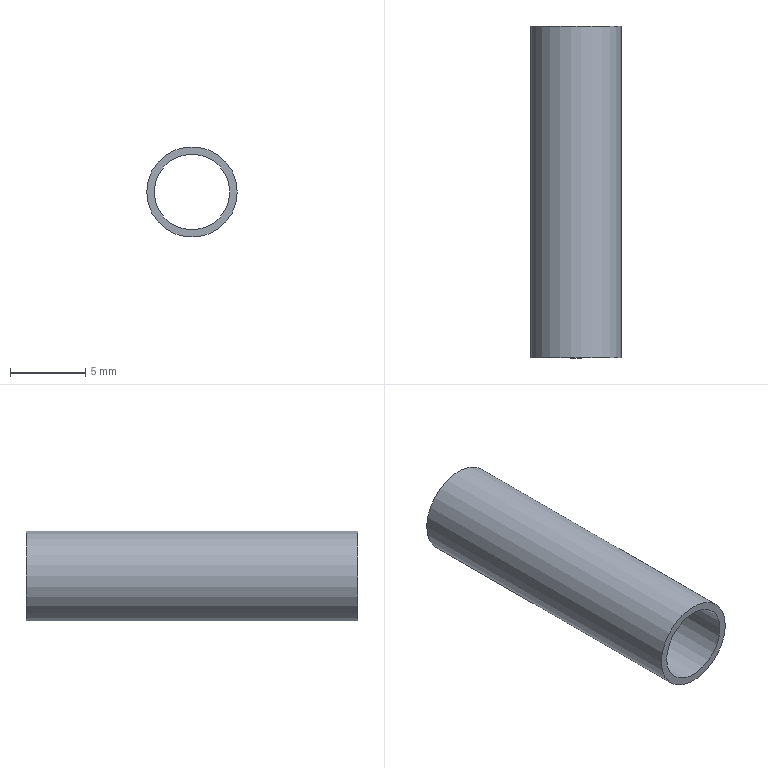Part | STEP file | 1-73.9 | 1 solid | 4 faces | box 6 x 22 x 6 mm | volume 190.066 mm3 | cylinder 2 | plane 2 | commonest cylinder face diameters 5 x1 6 x1
STEP:
#1=CARTESIAN_POINT('',(0.,0.,0.));
#2=DIRECTION('',(0.,0.,1.));
#3=DIRECTION('',(1.,0.,0.));
#4=AXIS2_PLACEMENT_3D('',#1,#2,#3);
#5=CARTESIAN_POINT('',(3.,0.,0.));
#6=VERTEX_POINT('',#5);
#7=CARTESIAN_POINT('',(0.,0.,0.));
#8=DIRECTION('',(0.,-1.,0.));
#9=DIRECTION('',(1.,0.,0.));
#10=AXIS2_PLACEMENT_3D('',#7,#8,#9);
#11=CIRCLE('',#10,3.);
#12=CARTESIAN_POINT('',(0.,0.,0.));
#13=DIRECTION('',(0.,1.,0.));
#14=DIRECTION('',(1.,0.,0.));
#15=AXIS2_PLACEMENT_3D('',#12,#13,#14);
#16=CYLINDRICAL_SURFACE('',#15,3.);
#17=CARTESIAN_POINT('',(6.283,0.));
#18=DIRECTION('',(-1.,0.));
#19=VECTOR('',#18,1.);
#20=LINE('',#17,#19);
#21=(GEOMETRIC_REPRESENTATION_CONTEXT(2)PARAMETRIC_REPRESENTATION_CONTEXT()REPRESENTATION_CONTEXT('',''));
#22=DEFINITIONAL_REPRESENTATION('',(#20),#21);
#23=PCURVE('',#16,#22);
#24=CARTESIAN_POINT('',(0.,0.,0.));
#25=DIRECTION('',(0.,-1.,0.));
#26=DIRECTION('',(0.,0.,-1.));
#27=AXIS2_PLACEMENT_3D('',#24,#25,#26);
#28=PLANE('',#27);
#29=CARTESIAN_POINT('',(0.,0.));
#30=DIRECTION('',(0.,1.));
#31=AXIS2_PLACEMENT_2D('',#29,#30);
#32=CIRCLE('',#31,3.);
#33=(GEOMETRIC_REPRESENTATION_CONTEXT(2)PARAMETRIC_REPRESENTATION_CONTEXT()REPRESENTATION_CONTEXT('',''));
#34=DEFINITIONAL_REPRESENTATION('',(#32),#33);
#35=PCURVE('',#28,#34);
#36=SURFACE_CURVE('',#11,(#23,#35),.PCURVE_S1.);
#37=EDGE_CURVE('',#6,#6,#36,.T.);
#38=ORIENTED_EDGE('',*,*,#37,.F.);
#39=CARTESIAN_POINT('',(3.,22.,0.));
#40=VERTEX_POINT('',#39);
#41=CARTESIAN_POINT('',(3.,0.,0.));
#42=DIRECTION('',(0.,1.,0.));
#43=VECTOR('',#42,1.);
#44=LINE('',#41,#43);
#45=CARTESIAN_POINT('',(6.283,0.));
#46=DIRECTION('',(0.,1.));
#47=VECTOR('',#46,1.);
#48=LINE('',#45,#47);
#49=(GEOMETRIC_REPRESENTATION_CONTEXT(2)PARAMETRIC_REPRESENTATION_CONTEXT()REPRESENTATION_CONTEXT('',''));
#50=DEFINITIONAL_REPRESENTATION('',(#48),#49);
#51=PCURVE('',#16,#50);
#52=CARTESIAN_POINT('',(0.,0.));
#53=DIRECTION('',(0.,1.));
#54=VECTOR('',#53,1.);
#55=LINE('',#52,#54);
#56=(GEOMETRIC_REPRESENTATION_CONTEXT(2)PARAMETRIC_REPRESENTATION_CONTEXT()REPRESENTATION_CONTEXT('',''));
#57=DEFINITIONAL_REPRESENTATION('',(#55),#56);
#58=PCURVE('',#16,#57);
#59=SEAM_CURVE('',#44,(#51,#58),.PCURVE_S1.);
#60=EDGE_CURVE('',#6,#40,#59,.T.);
#61=ORIENTED_EDGE('',*,*,#60,.T.);
#62=CARTESIAN_POINT('',(0.,22.,0.));
#63=DIRECTION('',(0.,1.,0.));
#64=DIRECTION('',(1.,0.,0.));
#65=AXIS2_PLACEMENT_3D('',#62,#63,#64);
#66=CIRCLE('',#65,3.);
#67=CARTESIAN_POINT('',(0.,22.));
#68=DIRECTION('',(1.,0.));
#69=VECTOR('',#68,1.);
#70=LINE('',#67,#69);
#71=(GEOMETRIC_REPRESENTATION_CONTEXT(2)PARAMETRIC_REPRESENTATION_CONTEXT()REPRESENTATION_CONTEXT('',''));
#72=DEFINITIONAL_REPRESENTATION('',(#70),#71);
#73=PCURVE('',#16,#72);
#74=CARTESIAN_POINT('',(0.,22.,0.));
#75=DIRECTION('',(0.,1.,0.));
#76=DIRECTION('',(0.,0.,1.));
#77=AXIS2_PLACEMENT_3D('',#74,#75,#76);
#78=PLANE('',#77);
#79=CARTESIAN_POINT('',(0.,0.));
#80=DIRECTION('',(0.,1.));
#81=AXIS2_PLACEMENT_2D('',#79,#80);
#82=CIRCLE('',#81,3.);
#83=(GEOMETRIC_REPRESENTATION_CONTEXT(2)PARAMETRIC_REPRESENTATION_CONTEXT()REPRESENTATION_CONTEXT('',''));
#84=DEFINITIONAL_REPRESENTATION('',(#82),#83);
#85=PCURVE('',#78,#84);
#86=SURFACE_CURVE('',#66,(#73,#85),.PCURVE_S1.);
#87=EDGE_CURVE('',#40,#40,#86,.T.);
#88=ORIENTED_EDGE('',*,*,#87,.F.);
#89=ORIENTED_EDGE('',*,*,#60,.F.);
#90=EDGE_LOOP('',(#38,#61,#88,#89));
#91=FACE_BOUND('',#90,.T.);
#92=ADVANCED_FACE('',(#91),#16,.T.);
#93=ORIENTED_EDGE('',*,*,#37,.T.);
#94=EDGE_LOOP('',(#93));
#95=FACE_BOUND('',#94,.T.);
#96=CARTESIAN_POINT('',(2.5,0.,0.));
#97=VERTEX_POINT('',#96);
#98=CARTESIAN_POINT('',(0.,0.,0.));
#99=DIRECTION('',(0.,-1.,0.));
#100=DIRECTION('',(1.,0.,0.));
#101=AXIS2_PLACEMENT_3D('',#98,#99,#100);
#102=CIRCLE('',#101,2.5);
#103=CARTESIAN_POINT('',(0.,0.));
#104=DIRECTION('',(0.,1.));
#105=AXIS2_PLACEMENT_2D('',#103,#104);
#106=CIRCLE('',#105,2.5);
#107=(GEOMETRIC_REPRESENTATION_CONTEXT(2)PARAMETRIC_REPRESENTATION_CONTEXT()REPRESENTATION_CONTEXT('',''));
#108=DEFINITIONAL_REPRESENTATION('',(#106),#107);
#109=PCURVE('',#28,#108);
#110=CARTESIAN_POINT('',(0.,0.,0.));
#111=DIRECTION('',(0.,1.,0.));
#112=DIRECTION('',(1.,0.,0.));
#113=AXIS2_PLACEMENT_3D('',#110,#111,#112);
#114=CYLINDRICAL_SURFACE('',#113,2.5);
#115=CARTESIAN_POINT('',(6.283,0.));
#116=DIRECTION('',(-1.,0.));
#117=VECTOR('',#116,1.);
#118=LINE('',#115,#117);
#119=(GEOMETRIC_REPRESENTATION_CONTEXT(2)PARAMETRIC_REPRESENTATION_CONTEXT()REPRESENTATION_CONTEXT('',''));
#120=DEFINITIONAL_REPRESENTATION('',(#118),#119);
#121=PCURVE('',#114,#120);
#122=SURFACE_CURVE('',#102,(#109,#121),.PCURVE_S1.);
#123=EDGE_CURVE('',#97,#97,#122,.T.);
#124=ORIENTED_EDGE('',*,*,#123,.F.);
#125=EDGE_LOOP('',(#124));
#126=FACE_BOUND('',#125,.T.);
#127=ADVANCED_FACE('',(#95,#126),#28,.T.);
#128=ORIENTED_EDGE('',*,*,#87,.T.);
#129=EDGE_LOOP('',(#128));
#130=FACE_BOUND('',#129,.T.);
#131=CARTESIAN_POINT('',(2.5,22.,0.));
#132=VERTEX_POINT('',#131);
#133=CARTESIAN_POINT('',(0.,22.,0.));
#134=DIRECTION('',(0.,1.,0.));
#135=DIRECTION('',(1.,0.,0.));
#136=AXIS2_PLACEMENT_3D('',#133,#134,#135);
#137=CIRCLE('',#136,2.5);
#138=CARTESIAN_POINT('',(0.,0.));
#139=DIRECTION('',(0.,1.));
#140=AXIS2_PLACEMENT_2D('',#138,#139);
#141=CIRCLE('',#140,2.5);
#142=(GEOMETRIC_REPRESENTATION_CONTEXT(2)PARAMETRIC_REPRESENTATION_CONTEXT()REPRESENTATION_CONTEXT('',''));
#143=DEFINITIONAL_REPRESENTATION('',(#141),#142);
#144=PCURVE('',#78,#143);
#145=CARTESIAN_POINT('',(0.,22.));
#146=DIRECTION('',(1.,0.));
#147=VECTOR('',#146,1.);
#148=LINE('',#145,#147);
#149=(GEOMETRIC_REPRESENTATION_CONTEXT(2)PARAMETRIC_REPRESENTATION_CONTEXT()REPRESENTATION_CONTEXT('',''));
#150=DEFINITIONAL_REPRESENTATION('',(#148),#149);
#151=PCURVE('',#114,#150);
#152=SURFACE_CURVE('',#137,(#144,#151),.PCURVE_S1.);
#153=EDGE_CURVE('',#132,#132,#152,.T.);
#154=ORIENTED_EDGE('',*,*,#153,.F.);
#155=EDGE_LOOP('',(#154));
#156=FACE_BOUND('',#155,.T.);
#157=ADVANCED_FACE('',(#130,#156),#78,.T.);
#158=ORIENTED_EDGE('',*,*,#123,.F.);
#159=CARTESIAN_POINT('',(2.5,0.,0.));
#160=DIRECTION('',(0.,1.,0.));
#161=VECTOR('',#160,1.);
#162=LINE('',#159,#161);
#163=CARTESIAN_POINT('',(6.283,0.));
#164=DIRECTION('',(0.,1.));
#165=VECTOR('',#164,1.);
#166=LINE('',#163,#165);
#167=(GEOMETRIC_REPRESENTATION_CONTEXT(2)PARAMETRIC_REPRESENTATION_CONTEXT()REPRESENTATION_CONTEXT('',''));
#168=DEFINITIONAL_REPRESENTATION('',(#166),#167);
#169=PCURVE('',#114,#168);
#170=CARTESIAN_POINT('',(0.,0.));
#171=DIRECTION('',(0.,1.));
#172=VECTOR('',#171,1.);
#173=LINE('',#170,#172);
#174=(GEOMETRIC_REPRESENTATION_CONTEXT(2)PARAMETRIC_REPRESENTATION_CONTEXT()REPRESENTATION_CONTEXT('',''));
#175=DEFINITIONAL_REPRESENTATION('',(#173),#174);
#176=PCURVE('',#114,#175);
#177=SEAM_CURVE('',#162,(#169,#176),.PCURVE_S1.);
#178=EDGE_CURVE('',#97,#132,#177,.T.);
#179=ORIENTED_EDGE('',*,*,#178,.T.);
#180=ORIENTED_EDGE('',*,*,#153,.F.);
#181=ORIENTED_EDGE('',*,*,#178,.F.);
#182=EDGE_LOOP('',(#158,#179,#180,#181));
#183=FACE_BOUND('',#182,.F.);
#184=ADVANCED_FACE('',(#183),#114,.F.);
#185=CLOSED_SHELL('',(#92,#127,#157,#184));
#186=MANIFOLD_SOLID_BREP('',#185);
#187=(LENGTH_UNIT()NAMED_UNIT(*)SI_UNIT(.MILLI.,.METRE.));
#188=UNCERTAINTY_MEASURE_WITH_UNIT(LENGTH_MEASURE(0.0000001),#187,'','');
#189=(NAMED_UNIT(*)PLANE_ANGLE_UNIT()SI_UNIT($,.RADIAN.));
#190=(NAMED_UNIT(*)SI_UNIT($,.STERADIAN.)SOLID_ANGLE_UNIT());
#191=(GEOMETRIC_REPRESENTATION_CONTEXT(3)GLOBAL_UNCERTAINTY_ASSIGNED_CONTEXT((#188))GLOBAL_UNIT_ASSIGNED_CONTEXT((#187,#189,#190))REPRESENTATION_CONTEXT('',''));
#192=ADVANCED_BREP_SHAPE_REPRESENTATION('',(#4,#186),#191);